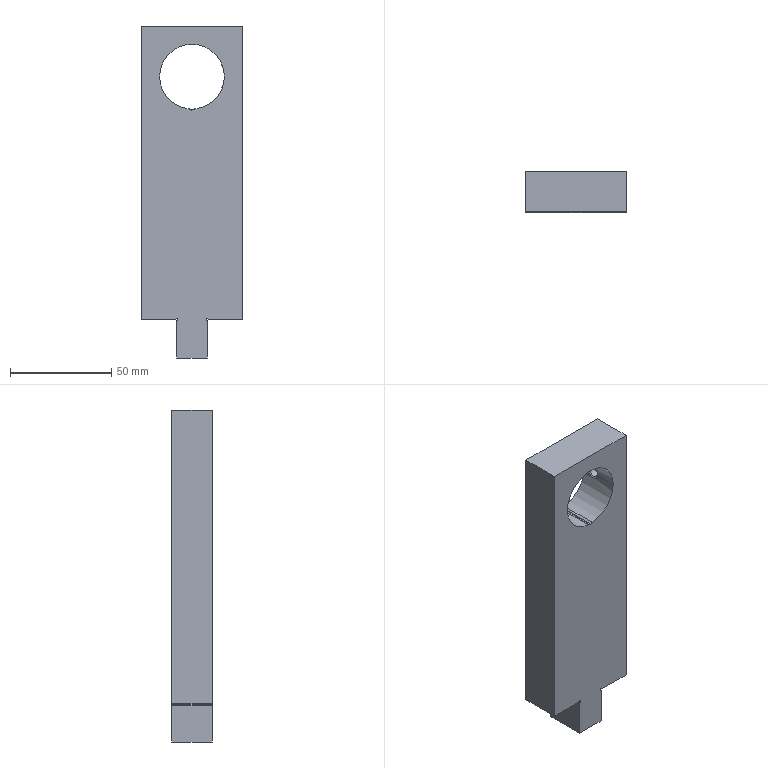Part | STEP file | YBQDJ-DX-2 | 1 solid | 23 faces | box 50 x 20 x 164 mm | volume 134384 mm3 | cylinder 11 | plane 10 | cone 1 | spline 1 | commonest cylinder face diameters 2 x4 1 x3 4 x2 5 x1 32.01 x1